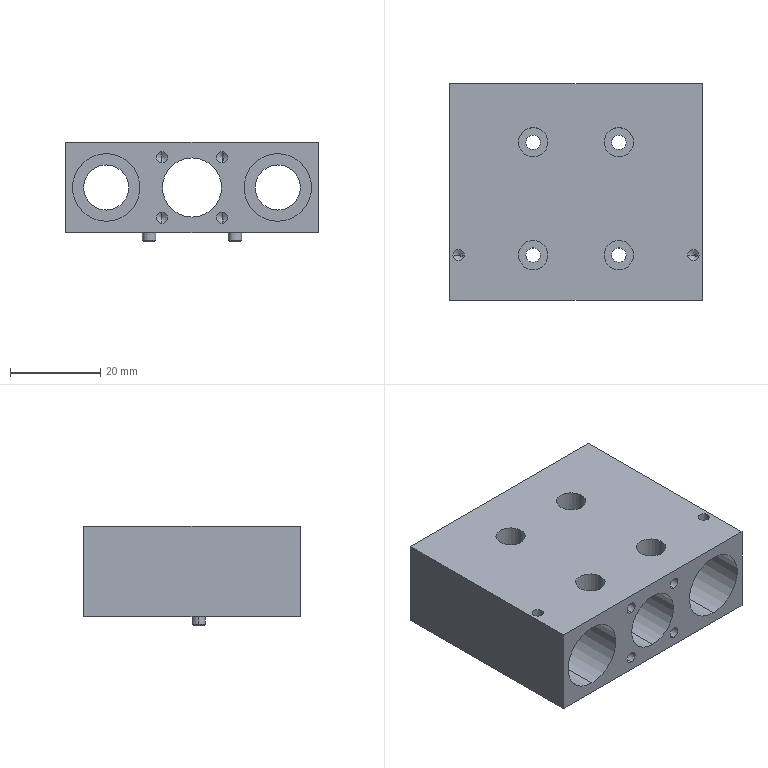NC program | NX | posted with a generic post | part box 56 x 48 x 22 mm
Whole program:
N10 G17 G21 G94 G90
(FLOOR_WALL_COPY , TOOL : D63)
N12 T01 M6
N14 G54
N16 G17 G0 G90 X64.5 Y0. B0. C0. S6500 M3
N18 G43 Z30. H1
N20 Z5.
N22 G94 G1 Z2. F1500.
N24 X59.5
N26 X-59.5
N28 X-64.5
N30 Z5.
N32 G0 Z30.
N34 X64.5
N36 Z4.
N38 G1 Z1.
N40 X59.5
N42 X-59.5
N44 X-64.5
N46 Z4.
N48 G0 Z30.
N50 X64.5
N52 Z3.
N54 G1 Z0.
N56 X59.5
N58 X-59.5
N60 X-64.5
N62 Z3.
N64 G0 Z30.
N66 M5
(FLOOR_WALL_1_COPY , TOOL : D10)
N68 T10 M6
N70 G54
N72 G17 G0 G90 X34.5 Y-25.595 B0. C0. S9500 M3
N74 G43 Z30. H10
N76 Z-0.5
N78 G94 G1 Z-2. F1000.
N80 X33.866 Y-24.497
N82 G3 X33. Y-23.997 R1.
N84 G1 X-33. F1500.
N86 Y-19.108
N88 X33.
N90 Y-14.22
N92 X-33.
N94 Y-9.331
N96 X33.
N98 Y-4.443
N100 X13.199
N102 G3 X16.42 Y0.446 R7.
N104 G1 X33.
N106 Y5.334
N108 X15.356
N110 G3 X16.249 Y4.884 R1.
N112 G1 Z-0.5
N114 G0 Z30.
N116 X13.199 Y-4.443
N118 Z-0.5
N120 G1 Z-2. F1000.
N122 G2 X5.801 Y-4.443 R7.
N124 G1 X-5.801 F1500.
N126 G3 X-2.58 Y0.446 R7.
N128 G1 X2.58
N130 G2 X3.644 Y5.334 R7.
N132 G1 X-3.644
N134 G3 X-2.751 Y4.884 R1.
N136 G1 Z-0.5
N138 G0 Z30.
N140 X-5.801 Y-4.443
N142 Z-0.5
N144 G1 Z-2. F1000.
N146 G2 X-13.199 Y-4.443 R7.
N148 G1 X-33. F1500.
N150 Y0.446
N152 X-16.42
N154 G2 X-15.356 Y5.334 R7.
N156 G1 X-33.
N158 Y10.223
N160 X33.
N162 Y15.111
N164 X-33.
N166 Y20.
N168 X33.
N170 G2 X33.866 Y19.5 R1.
N172 G1 X34.5 Y18.402
N174 Z-0.5
N176 G0 X17.84 Y3.14
N178 G1 Z-2. F1000.
N180 X16.5 Y2.366
N182 G3 X16. Y1.5 R1.
N184 G2 X9.5 Y-5. R6.5 F1500.
N186 X16. Y1.5 R-6.5
N188 G3 X16.5 Y0.634 R1.
N190 G1 X17.84 Y-0.14
N192 Z-0.5
N194 G0 Z30.
N196 X-17.84
N198 Z-0.5
N200 G1 Z-2. F1000.
N202 X-16.5 Y0.634
N204 G3 X-16. Y1.5 R1.
N206 G2 X-9.5 Y8. R6.5 F1500.
N208 X-16. Y1.5 R-6.5
N210 G3 X-16.5 Y2.366 R1.
N212 G1 X-17.84 Y3.14
N214 Z-0.5
N216 G0 Z30.
N218 M5
(PLANAR_MILL_COPY_1 , TOOL : D6A45)
N220 T07 M6
N222 G54
N224 G17 G0 G90 X-9.883 Y-11.521 B0. C0. S9500 M3
N226 G43 Z30. H7
N228 Z0.
N230 G94 G1 Z-3. F1250.
N232 G3 X-9.5 Y-11.7 R0.5
N234 X-8.8 Y-11. R0.7
N236 X-9.5 Y-11.7 R-0.7
N238 X-9.117 Y-11.521 R0.5
N240 G1 Z0.
N242 G0 Z30.
N244 X9.117
N246 Z0.
N248 G1 Z-3.
N250 G3 X9.5 Y-11.7 R0.5
N252 X10.2 Y-11. R0.7
N254 X9.5 Y-11.7 R-0.7
N256 X9.883 Y-11.521 R0.5
N258 G1 Z0.
N260 G0 Z30.
N262 X0.766 Y-25.257
N264 Z0.
N266 G1 Z-3.
N268 G3 X0. Y-24.9 R1.
N270 G1 X-28.
N272 G2 X-28.9 Y-24. R0.9
N274 G1 Y24.
N276 G2 X-28. Y24.9 R0.9
N278 G1 X28.
N280 G2 X28.9 Y24. R0.9
N282 G1 Y-24.
N284 G2 X28. Y-24.9 R0.9
N286 G1 X0.
N288 G3 X-0.766 Y-25.257 R1.
N290 G1 Z0.
N292 G0 Z30.
N294 X9.883 Y14.521
N296 Z0.
N298 G1 Z-3.
N300 G3 X9.5 Y14.7 R0.5
N302 X8.8 Y14. R0.7
N304 X9.5 Y14.7 R-0.7
N306 X9.117 Y14.521 R0.5
N308 G1 Z0.
N310 G0 Z30.
N312 X-9.117
N314 Z0.
N316 G1 Z-3.
N318 G3 X-9.5 Y14.7 R0.5
N320 X-10.2 Y14. R0.7
N322 X-9.5 Y14.7 R-0.7
N324 X-9.883 Y14.521 R0.5
N326 G1 Z0.
N328 G0 Z30.
N330 M5
N332 M2